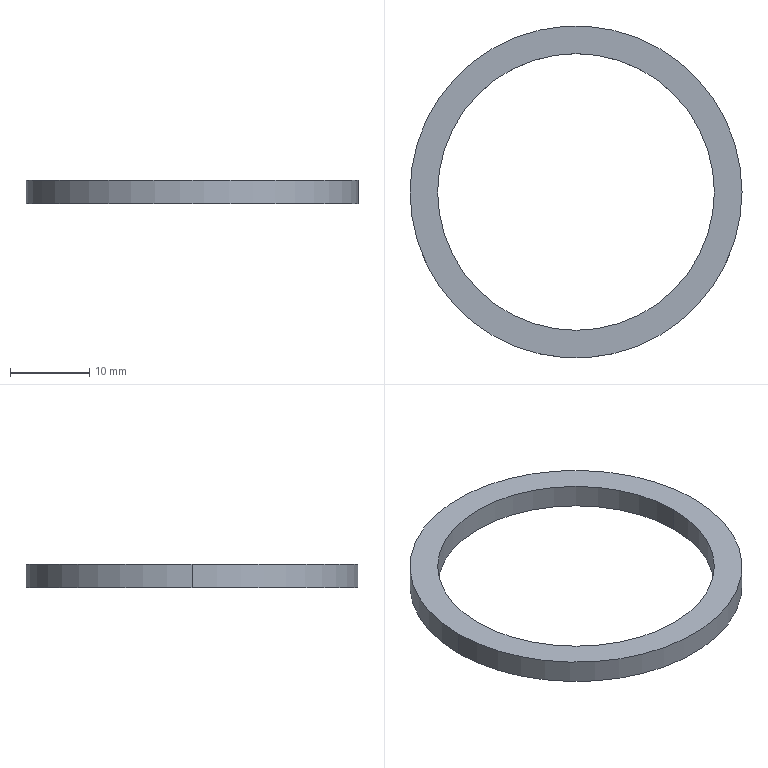Part | STEP file | 02-Spacer 2 | 1 solid | 6 faces | box 42 x 42 x 3 mm | volume 1270 mm3 | cylinder 4 | plane 2 | commonest cylinder face diameters 35 x2 42 x2
STEP:
#1=CARTESIAN_POINT('',(0.,0.,0.));
#2=DIRECTION('',(0.,0.,1.));
#3=DIRECTION('',(1.,0.,0.));
#4=AXIS2_PLACEMENT_3D('',#1,#2,#3);
#5=CARTESIAN_POINT('',(-17.5,0.,3.));
#6=VERTEX_POINT('',#5);
#7=CARTESIAN_POINT('',(-17.5,0.,0.));
#8=VERTEX_POINT('',#7);
#9=CARTESIAN_POINT('',(-17.5,0.,3.));
#10=DIRECTION('',(0.,0.,-1.));
#11=VECTOR('',#10,1.);
#12=LINE('',#9,#11);
#13=CARTESIAN_POINT('',(0.,0.,3.));
#14=DIRECTION('',(0.,0.,-1.));
#15=DIRECTION('',(-1.,0.,0.));
#16=AXIS2_PLACEMENT_3D('',#13,#14,#15);
#17=CYLINDRICAL_SURFACE('',#16,17.5);
#18=CARTESIAN_POINT('',(6.283,0.));
#19=DIRECTION('',(0.,1.));
#20=VECTOR('',#19,1.);
#21=LINE('',#18,#20);
#22=(GEOMETRIC_REPRESENTATION_CONTEXT(2)PARAMETRIC_REPRESENTATION_CONTEXT()REPRESENTATION_CONTEXT('',''));
#23=DEFINITIONAL_REPRESENTATION('',(#21),#22);
#24=PCURVE('',#17,#23);
#25=CARTESIAN_POINT('',(0.,0.,3.));
#26=DIRECTION('',(0.,0.,-1.));
#27=DIRECTION('',(-1.,0.,0.));
#28=AXIS2_PLACEMENT_3D('',#25,#26,#27);
#29=CYLINDRICAL_SURFACE('',#28,17.5);
#30=CARTESIAN_POINT('',(0.,0.));
#31=DIRECTION('',(0.,1.));
#32=VECTOR('',#31,1.);
#33=LINE('',#30,#32);
#34=(GEOMETRIC_REPRESENTATION_CONTEXT(2)PARAMETRIC_REPRESENTATION_CONTEXT()REPRESENTATION_CONTEXT('',''));
#35=DEFINITIONAL_REPRESENTATION('',(#33),#34);
#36=PCURVE('',#29,#35);
#37=SURFACE_CURVE('',#12,(#24,#36),.PCURVE_S1.);
#38=EDGE_CURVE('',#6,#8,#37,.T.);
#39=ORIENTED_EDGE('',*,*,#38,.T.);
#40=CARTESIAN_POINT('',(17.5,0.,0.));
#41=VERTEX_POINT('',#40);
#42=CARTESIAN_POINT('',(0.,0.,0.));
#43=DIRECTION('',(0.,0.,1.));
#44=DIRECTION('',(1.,0.,0.));
#45=AXIS2_PLACEMENT_3D('',#42,#43,#44);
#46=CIRCLE('',#45,17.5);
#47=CARTESIAN_POINT('',(9.425,3.));
#48=DIRECTION('',(-1.,0.));
#49=VECTOR('',#48,1.);
#50=LINE('',#47,#49);
#51=(GEOMETRIC_REPRESENTATION_CONTEXT(2)PARAMETRIC_REPRESENTATION_CONTEXT()REPRESENTATION_CONTEXT('',''));
#52=DEFINITIONAL_REPRESENTATION('',(#50),#51);
#53=PCURVE('',#17,#52);
#54=CARTESIAN_POINT('',(0.,0.,0.));
#55=DIRECTION('',(0.,0.,1.));
#56=DIRECTION('',(1.,0.,0.));
#57=AXIS2_PLACEMENT_3D('',#54,#55,#56);
#58=PLANE('',#57);
#59=CARTESIAN_POINT('',(0.,0.));
#60=DIRECTION('',(1.,0.));
#61=AXIS2_PLACEMENT_2D('',#59,#60);
#62=CIRCLE('',#61,17.5);
#63=(GEOMETRIC_REPRESENTATION_CONTEXT(2)PARAMETRIC_REPRESENTATION_CONTEXT()REPRESENTATION_CONTEXT('',''));
#64=DEFINITIONAL_REPRESENTATION('',(#62),#63);
#65=PCURVE('',#58,#64);
#66=SURFACE_CURVE('',#46,(#53,#65),.PCURVE_S1.);
#67=EDGE_CURVE('',#8,#41,#66,.T.);
#68=ORIENTED_EDGE('',*,*,#67,.T.);
#69=CARTESIAN_POINT('',(17.5,0.,3.));
#70=VERTEX_POINT('',#69);
#71=CARTESIAN_POINT('',(17.5,0.,3.));
#72=DIRECTION('',(0.,0.,-1.));
#73=VECTOR('',#72,1.);
#74=LINE('',#71,#73);
#75=CARTESIAN_POINT('',(3.142,0.));
#76=DIRECTION('',(0.,1.));
#77=VECTOR('',#76,1.);
#78=LINE('',#75,#77);
#79=(GEOMETRIC_REPRESENTATION_CONTEXT(2)PARAMETRIC_REPRESENTATION_CONTEXT()REPRESENTATION_CONTEXT('',''));
#80=DEFINITIONAL_REPRESENTATION('',(#78),#79);
#81=PCURVE('',#17,#80);
#82=CARTESIAN_POINT('',(3.142,0.));
#83=DIRECTION('',(0.,1.));
#84=VECTOR('',#83,1.);
#85=LINE('',#82,#84);
#86=(GEOMETRIC_REPRESENTATION_CONTEXT(2)PARAMETRIC_REPRESENTATION_CONTEXT()REPRESENTATION_CONTEXT('',''));
#87=DEFINITIONAL_REPRESENTATION('',(#85),#86);
#88=PCURVE('',#29,#87);
#89=SURFACE_CURVE('',#74,(#81,#88),.PCURVE_S1.);
#90=EDGE_CURVE('',#70,#41,#89,.T.);
#91=ORIENTED_EDGE('',*,*,#90,.F.);
#92=CARTESIAN_POINT('',(0.,0.,3.));
#93=DIRECTION('',(0.,0.,1.));
#94=DIRECTION('',(1.,0.,0.));
#95=AXIS2_PLACEMENT_3D('',#92,#93,#94);
#96=CIRCLE('',#95,17.5);
#97=CARTESIAN_POINT('',(9.425,0.));
#98=DIRECTION('',(-1.,0.));
#99=VECTOR('',#98,1.);
#100=LINE('',#97,#99);
#101=(GEOMETRIC_REPRESENTATION_CONTEXT(2)PARAMETRIC_REPRESENTATION_CONTEXT()REPRESENTATION_CONTEXT('',''));
#102=DEFINITIONAL_REPRESENTATION('',(#100),#101);
#103=PCURVE('',#17,#102);
#104=CARTESIAN_POINT('',(0.,0.,3.));
#105=DIRECTION('',(0.,0.,1.));
#106=DIRECTION('',(1.,0.,0.));
#107=AXIS2_PLACEMENT_3D('',#104,#105,#106);
#108=PLANE('',#107);
#109=CARTESIAN_POINT('',(0.,0.));
#110=DIRECTION('',(1.,0.));
#111=AXIS2_PLACEMENT_2D('',#109,#110);
#112=CIRCLE('',#111,17.5);
#113=(GEOMETRIC_REPRESENTATION_CONTEXT(2)PARAMETRIC_REPRESENTATION_CONTEXT()REPRESENTATION_CONTEXT('',''));
#114=DEFINITIONAL_REPRESENTATION('',(#112),#113);
#115=PCURVE('',#108,#114);
#116=SURFACE_CURVE('',#96,(#103,#115),.PCURVE_S1.);
#117=EDGE_CURVE('',#6,#70,#116,.T.);
#118=ORIENTED_EDGE('',*,*,#117,.F.);
#119=EDGE_LOOP('',(#39,#68,#91,#118));
#120=FACE_BOUND('',#119,.F.);
#121=ADVANCED_FACE('',(#120),#17,.F.);
#122=CARTESIAN_POINT('',(21.,0.,3.));
#123=VERTEX_POINT('',#122);
#124=CARTESIAN_POINT('',(-21.,0.,3.));
#125=VERTEX_POINT('',#124);
#126=CARTESIAN_POINT('',(0.,0.,3.));
#127=DIRECTION('',(0.,0.,1.));
#128=DIRECTION('',(1.,0.,0.));
#129=AXIS2_PLACEMENT_3D('',#126,#127,#128);
#130=CIRCLE('',#129,21.);
#131=CARTESIAN_POINT('',(0.,0.,3.));
#132=DIRECTION('',(0.,0.,-1.));
#133=DIRECTION('',(-1.,0.,0.));
#134=AXIS2_PLACEMENT_3D('',#131,#132,#133);
#135=CYLINDRICAL_SURFACE('',#134,21.);
#136=CARTESIAN_POINT('',(3.142,0.));
#137=DIRECTION('',(-1.,0.));
#138=VECTOR('',#137,1.);
#139=LINE('',#136,#138);
#140=(GEOMETRIC_REPRESENTATION_CONTEXT(2)PARAMETRIC_REPRESENTATION_CONTEXT()REPRESENTATION_CONTEXT('',''));
#141=DEFINITIONAL_REPRESENTATION('',(#139),#140);
#142=PCURVE('',#135,#141);
#143=CARTESIAN_POINT('',(0.,0.));
#144=DIRECTION('',(1.,0.));
#145=AXIS2_PLACEMENT_2D('',#143,#144);
#146=CIRCLE('',#145,21.);
#147=(GEOMETRIC_REPRESENTATION_CONTEXT(2)PARAMETRIC_REPRESENTATION_CONTEXT()REPRESENTATION_CONTEXT('',''));
#148=DEFINITIONAL_REPRESENTATION('',(#146),#147);
#149=PCURVE('',#108,#148);
#150=SURFACE_CURVE('',#130,(#142,#149),.PCURVE_S1.);
#151=EDGE_CURVE('',#123,#125,#150,.T.);
#152=ORIENTED_EDGE('',*,*,#151,.F.);
#153=CARTESIAN_POINT('',(21.,0.,0.));
#154=VERTEX_POINT('',#153);
#155=CARTESIAN_POINT('',(21.,0.,3.));
#156=DIRECTION('',(0.,0.,-1.));
#157=VECTOR('',#156,1.);
#158=LINE('',#155,#157);
#159=CARTESIAN_POINT('',(3.142,0.));
#160=DIRECTION('',(0.,1.));
#161=VECTOR('',#160,1.);
#162=LINE('',#159,#161);
#163=(GEOMETRIC_REPRESENTATION_CONTEXT(2)PARAMETRIC_REPRESENTATION_CONTEXT()REPRESENTATION_CONTEXT('',''));
#164=DEFINITIONAL_REPRESENTATION('',(#162),#163);
#165=PCURVE('',#135,#164);
#166=CARTESIAN_POINT('',(0.,0.,3.));
#167=DIRECTION('',(0.,0.,-1.));
#168=DIRECTION('',(-1.,0.,0.));
#169=AXIS2_PLACEMENT_3D('',#166,#167,#168);
#170=CYLINDRICAL_SURFACE('',#169,21.);
#171=CARTESIAN_POINT('',(3.142,0.));
#172=DIRECTION('',(0.,1.));
#173=VECTOR('',#172,1.);
#174=LINE('',#171,#173);
#175=(GEOMETRIC_REPRESENTATION_CONTEXT(2)PARAMETRIC_REPRESENTATION_CONTEXT()REPRESENTATION_CONTEXT('',''));
#176=DEFINITIONAL_REPRESENTATION('',(#174),#175);
#177=PCURVE('',#170,#176);
#178=SURFACE_CURVE('',#158,(#165,#177),.PCURVE_S1.);
#179=EDGE_CURVE('',#123,#154,#178,.T.);
#180=ORIENTED_EDGE('',*,*,#179,.T.);
#181=CARTESIAN_POINT('',(-21.,0.,0.));
#182=VERTEX_POINT('',#181);
#183=CARTESIAN_POINT('',(0.,0.,0.));
#184=DIRECTION('',(0.,0.,1.));
#185=DIRECTION('',(1.,0.,0.));
#186=AXIS2_PLACEMENT_3D('',#183,#184,#185);
#187=CIRCLE('',#186,21.);
#188=CARTESIAN_POINT('',(3.142,3.));
#189=DIRECTION('',(-1.,0.));
#190=VECTOR('',#189,1.);
#191=LINE('',#188,#190);
#192=(GEOMETRIC_REPRESENTATION_CONTEXT(2)PARAMETRIC_REPRESENTATION_CONTEXT()REPRESENTATION_CONTEXT('',''));
#193=DEFINITIONAL_REPRESENTATION('',(#191),#192);
#194=PCURVE('',#135,#193);
#195=CARTESIAN_POINT('',(0.,0.));
#196=DIRECTION('',(1.,0.));
#197=AXIS2_PLACEMENT_2D('',#195,#196);
#198=CIRCLE('',#197,21.);
#199=(GEOMETRIC_REPRESENTATION_CONTEXT(2)PARAMETRIC_REPRESENTATION_CONTEXT()REPRESENTATION_CONTEXT('',''));
#200=DEFINITIONAL_REPRESENTATION('',(#198),#199);
#201=PCURVE('',#58,#200);
#202=SURFACE_CURVE('',#187,(#194,#201),.PCURVE_S1.);
#203=EDGE_CURVE('',#154,#182,#202,.T.);
#204=ORIENTED_EDGE('',*,*,#203,.T.);
#205=CARTESIAN_POINT('',(-21.,0.,3.));
#206=DIRECTION('',(0.,0.,-1.));
#207=VECTOR('',#206,1.);
#208=LINE('',#205,#207);
#209=CARTESIAN_POINT('',(0.,0.));
#210=DIRECTION('',(0.,1.));
#211=VECTOR('',#210,1.);
#212=LINE('',#209,#211);
#213=(GEOMETRIC_REPRESENTATION_CONTEXT(2)PARAMETRIC_REPRESENTATION_CONTEXT()REPRESENTATION_CONTEXT('',''));
#214=DEFINITIONAL_REPRESENTATION('',(#212),#213);
#215=PCURVE('',#135,#214);
#216=CARTESIAN_POINT('',(6.283,0.));
#217=DIRECTION('',(0.,1.));
#218=VECTOR('',#217,1.);
#219=LINE('',#216,#218);
#220=(GEOMETRIC_REPRESENTATION_CONTEXT(2)PARAMETRIC_REPRESENTATION_CONTEXT()REPRESENTATION_CONTEXT('',''));
#221=DEFINITIONAL_REPRESENTATION('',(#219),#220);
#222=PCURVE('',#170,#221);
#223=SURFACE_CURVE('',#208,(#215,#222),.PCURVE_S1.);
#224=EDGE_CURVE('',#125,#182,#223,.T.);
#225=ORIENTED_EDGE('',*,*,#224,.F.);
#226=EDGE_LOOP('',(#152,#180,#204,#225));
#227=FACE_BOUND('',#226,.T.);
#228=ADVANCED_FACE('',(#227),#135,.T.);
#229=CARTESIAN_POINT('',(0.,0.,3.));
#230=DIRECTION('',(0.,0.,1.));
#231=DIRECTION('',(1.,0.,0.));
#232=AXIS2_PLACEMENT_3D('',#229,#230,#231);
#233=CIRCLE('',#232,21.);
#234=CARTESIAN_POINT('',(0.,0.));
#235=DIRECTION('',(1.,0.));
#236=AXIS2_PLACEMENT_2D('',#234,#235);
#237=CIRCLE('',#236,21.);
#238=(GEOMETRIC_REPRESENTATION_CONTEXT(2)PARAMETRIC_REPRESENTATION_CONTEXT()REPRESENTATION_CONTEXT('',''));
#239=DEFINITIONAL_REPRESENTATION('',(#237),#238);
#240=PCURVE('',#108,#239);
#241=CARTESIAN_POINT('',(9.425,0.));
#242=DIRECTION('',(-1.,0.));
#243=VECTOR('',#242,1.);
#244=LINE('',#241,#243);
#245=(GEOMETRIC_REPRESENTATION_CONTEXT(2)PARAMETRIC_REPRESENTATION_CONTEXT()REPRESENTATION_CONTEXT('',''));
#246=DEFINITIONAL_REPRESENTATION('',(#244),#245);
#247=PCURVE('',#170,#246);
#248=SURFACE_CURVE('',#233,(#240,#247),.PCURVE_S1.);
#249=EDGE_CURVE('',#125,#123,#248,.T.);
#250=ORIENTED_EDGE('',*,*,#249,.T.);
#251=ORIENTED_EDGE('',*,*,#151,.T.);
#252=EDGE_LOOP('',(#250,#251));
#253=FACE_BOUND('',#252,.T.);
#254=ORIENTED_EDGE('',*,*,#117,.F.);
#255=CARTESIAN_POINT('',(0.,0.,3.));
#256=DIRECTION('',(0.,0.,1.));
#257=DIRECTION('',(1.,0.,0.));
#258=AXIS2_PLACEMENT_3D('',#255,#256,#257);
#259=CIRCLE('',#258,17.5);
#260=CARTESIAN_POINT('',(0.,0.));
#261=DIRECTION('',(1.,0.));
#262=AXIS2_PLACEMENT_2D('',#260,#261);
#263=CIRCLE('',#262,17.5);
#264=(GEOMETRIC_REPRESENTATION_CONTEXT(2)PARAMETRIC_REPRESENTATION_CONTEXT()REPRESENTATION_CONTEXT('',''));
#265=DEFINITIONAL_REPRESENTATION('',(#263),#264);
#266=PCURVE('',#108,#265);
#267=CARTESIAN_POINT('',(3.142,0.));
#268=DIRECTION('',(-1.,0.));
#269=VECTOR('',#268,1.);
#270=LINE('',#267,#269);
#271=(GEOMETRIC_REPRESENTATION_CONTEXT(2)PARAMETRIC_REPRESENTATION_CONTEXT()REPRESENTATION_CONTEXT('',''));
#272=DEFINITIONAL_REPRESENTATION('',(#270),#271);
#273=PCURVE('',#29,#272);
#274=SURFACE_CURVE('',#259,(#266,#273),.PCURVE_S1.);
#275=EDGE_CURVE('',#70,#6,#274,.T.);
#276=ORIENTED_EDGE('',*,*,#275,.F.);
#277=EDGE_LOOP('',(#254,#276));
#278=FACE_BOUND('',#277,.T.);
#279=ADVANCED_FACE('',(#253,#278),#108,.T.);
#280=CARTESIAN_POINT('',(0.,0.,0.));
#281=DIRECTION('',(0.,0.,1.));
#282=DIRECTION('',(1.,0.,0.));
#283=AXIS2_PLACEMENT_3D('',#280,#281,#282);
#284=CIRCLE('',#283,21.);
#285=CARTESIAN_POINT('',(0.,0.));
#286=DIRECTION('',(1.,0.));
#287=AXIS2_PLACEMENT_2D('',#285,#286);
#288=CIRCLE('',#287,21.);
#289=(GEOMETRIC_REPRESENTATION_CONTEXT(2)PARAMETRIC_REPRESENTATION_CONTEXT()REPRESENTATION_CONTEXT('',''));
#290=DEFINITIONAL_REPRESENTATION('',(#288),#289);
#291=PCURVE('',#58,#290);
#292=CARTESIAN_POINT('',(9.425,3.));
#293=DIRECTION('',(-1.,0.));
#294=VECTOR('',#293,1.);
#295=LINE('',#292,#294);
#296=(GEOMETRIC_REPRESENTATION_CONTEXT(2)PARAMETRIC_REPRESENTATION_CONTEXT()REPRESENTATION_CONTEXT('',''));
#297=DEFINITIONAL_REPRESENTATION('',(#295),#296);
#298=PCURVE('',#170,#297);
#299=SURFACE_CURVE('',#284,(#291,#298),.PCURVE_S1.);
#300=EDGE_CURVE('',#182,#154,#299,.T.);
#301=ORIENTED_EDGE('',*,*,#300,.F.);
#302=ORIENTED_EDGE('',*,*,#203,.F.);
#303=EDGE_LOOP('',(#301,#302));
#304=FACE_BOUND('',#303,.T.);
#305=ORIENTED_EDGE('',*,*,#67,.T.);
#306=CARTESIAN_POINT('',(0.,0.,0.));
#307=DIRECTION('',(0.,0.,1.));
#308=DIRECTION('',(1.,0.,0.));
#309=AXIS2_PLACEMENT_3D('',#306,#307,#308);
#310=CIRCLE('',#309,17.5);
#311=CARTESIAN_POINT('',(0.,0.));
#312=DIRECTION('',(1.,0.));
#313=AXIS2_PLACEMENT_2D('',#311,#312);
#314=CIRCLE('',#313,17.5);
#315=(GEOMETRIC_REPRESENTATION_CONTEXT(2)PARAMETRIC_REPRESENTATION_CONTEXT()REPRESENTATION_CONTEXT('',''));
#316=DEFINITIONAL_REPRESENTATION('',(#314),#315);
#317=PCURVE('',#58,#316);
#318=CARTESIAN_POINT('',(3.142,3.));
#319=DIRECTION('',(-1.,0.));
#320=VECTOR('',#319,1.);
#321=LINE('',#318,#320);
#322=(GEOMETRIC_REPRESENTATION_CONTEXT(2)PARAMETRIC_REPRESENTATION_CONTEXT()REPRESENTATION_CONTEXT('',''));
#323=DEFINITIONAL_REPRESENTATION('',(#321),#322);
#324=PCURVE('',#29,#323);
#325=SURFACE_CURVE('',#310,(#317,#324),.PCURVE_S1.);
#326=EDGE_CURVE('',#41,#8,#325,.T.);
#327=ORIENTED_EDGE('',*,*,#326,.T.);
#328=EDGE_LOOP('',(#305,#327));
#329=FACE_BOUND('',#328,.T.);
#330=ADVANCED_FACE('',(#304,#329),#58,.F.);
#331=ORIENTED_EDGE('',*,*,#179,.F.);
#332=ORIENTED_EDGE('',*,*,#249,.F.);
#333=ORIENTED_EDGE('',*,*,#224,.T.);
#334=ORIENTED_EDGE('',*,*,#300,.T.);
#335=EDGE_LOOP('',(#331,#332,#333,#334));
#336=FACE_BOUND('',#335,.T.);
#337=ADVANCED_FACE('',(#336),#170,.T.);
#338=ORIENTED_EDGE('',*,*,#326,.T.);
#339=ORIENTED_EDGE('',*,*,#38,.F.);
#340=ORIENTED_EDGE('',*,*,#275,.F.);
#341=ORIENTED_EDGE('',*,*,#90,.T.);
#342=EDGE_LOOP('',(#338,#339,#340,#341));
#343=FACE_BOUND('',#342,.F.);
#344=ADVANCED_FACE('',(#343),#29,.F.);
#345=CLOSED_SHELL('',(#121,#228,#279,#330,#337,#344));
#346=MANIFOLD_SOLID_BREP('',#345);
#347=(LENGTH_UNIT()NAMED_UNIT(*)SI_UNIT(.MILLI.,.METRE.));
#348=UNCERTAINTY_MEASURE_WITH_UNIT(LENGTH_MEASURE(0.0000001),#347,'','');
#349=(NAMED_UNIT(*)PLANE_ANGLE_UNIT()SI_UNIT($,.RADIAN.));
#350=(NAMED_UNIT(*)SI_UNIT($,.STERADIAN.)SOLID_ANGLE_UNIT());
#351=(GEOMETRIC_REPRESENTATION_CONTEXT(3)GLOBAL_UNCERTAINTY_ASSIGNED_CONTEXT((#348))GLOBAL_UNIT_ASSIGNED_CONTEXT((#347,#349,#350))REPRESENTATION_CONTEXT('',''));
#352=ADVANCED_BREP_SHAPE_REPRESENTATION('',(#4,#346),#351);